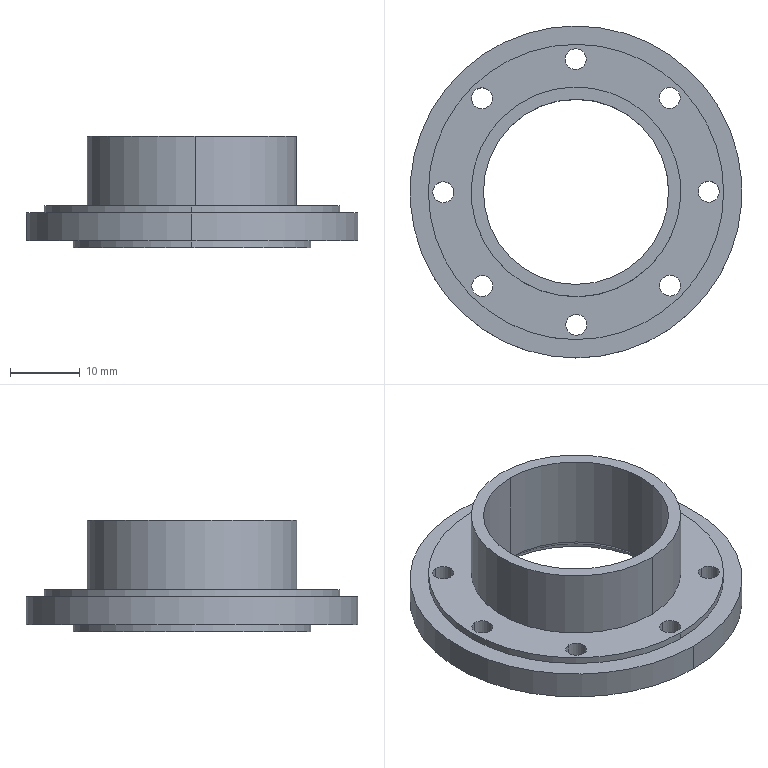Part | STEP file | 2026.6.15-Main Assembly图.sldasm-Part-105 | 1 solid | 36 faces | box 47.5 x 47.5 x 16 mm | volume 7161 mm3 | cylinder 28 | plane 6 | cone 2 | commonest cylinder face diameters 3 x16 30 x4 26.5 x2 34 x2 42.25 x2 47.5 x2
STEP:
#1=CARTESIAN_POINT('',(-1571.263,1411.006,3680.571));
#2=VERTEX_POINT('',#1);
#3=CARTESIAN_POINT('',(-1571.243,1437.506,3680.571));
#4=VERTEX_POINT('',#3);
#5=CARTESIAN_POINT('',(-1571.253,1424.256,3680.571));
#6=DIRECTION('',(0.,0.,-1.));
#7=DIRECTION('',(-0.0007664,-1.,0.));
#8=AXIS2_PLACEMENT_3D('',#5,#6,#7);
#9=CIRCLE('',#8,13.25);
#10=EDGE_CURVE('',#2,#4,#9,.T.);
#11=ORIENTED_EDGE('',*,*,#10,.F.);
#12=CARTESIAN_POINT('',(-1571.264,1410.006,3679.571));
#13=VERTEX_POINT('',#12);
#14=CARTESIAN_POINT('',(-1571.263,1411.006,3680.571));
#15=DIRECTION('',(-0.000542,-0.7071,-0.7071));
#16=VECTOR('',#15,1000.);
#17=LINE('',#14,#16);
#18=EDGE_CURVE('',#2,#13,#17,.T.);
#19=ORIENTED_EDGE('',*,*,#18,.T.);
#20=CARTESIAN_POINT('',(-1571.242,1438.506,3679.571));
#21=VERTEX_POINT('',#20);
#22=CARTESIAN_POINT('',(-1571.253,1424.256,3679.571));
#23=DIRECTION('',(0.,0.,1.));
#24=DIRECTION('',(-0.0007664,-1.,0.));
#25=AXIS2_PLACEMENT_3D('',#22,#23,#24);
#26=CIRCLE('',#25,14.25);
#27=EDGE_CURVE('',#21,#13,#26,.T.);
#28=ORIENTED_EDGE('',*,*,#27,.F.);
#29=CARTESIAN_POINT('',(-1571.243,1437.506,3680.571));
#30=DIRECTION('',(0.000542,0.7071,-0.7071));
#31=VECTOR('',#30,1000.);
#32=LINE('',#29,#31);
#33=EDGE_CURVE('',#4,#21,#32,.T.);
#34=ORIENTED_EDGE('',*,*,#33,.F.);
#35=EDGE_LOOP('',(#11,#19,#28,#34));
#36=FACE_OUTER_BOUND('',#35,.T.);
#37=CARTESIAN_POINT('',(-1571.253,1424.256,3680.571));
#38=DIRECTION('',(0.,0.,-1.));
#39=DIRECTION('',(0.0007664,1.,0.));
#40=AXIS2_PLACEMENT_3D('',#37,#38,#39);
#41=CONICAL_SURFACE('',#40,13.25,0.7854);
#42=ADVANCED_FACE('',(#36),#41,.F.);
#43=CARTESIAN_POINT('',(-1571.263,1411.006,3694.571));
#44=VERTEX_POINT('',#43);
#45=CARTESIAN_POINT('',(-1571.243,1437.506,3694.571));
#46=VERTEX_POINT('',#45);
#47=CARTESIAN_POINT('',(-1571.253,1424.256,3694.571));
#48=DIRECTION('',(0.,0.,-1.));
#49=DIRECTION('',(-0.0007664,-1.,0.));
#50=AXIS2_PLACEMENT_3D('',#47,#48,#49);
#51=CIRCLE('',#50,13.25);
#52=EDGE_CURVE('',#44,#46,#51,.T.);
#53=ORIENTED_EDGE('',*,*,#52,.F.);
#54=CARTESIAN_POINT('',(-1571.263,1411.006,3710.571));
#55=DIRECTION('',(0.,0.,-1.));
#56=VECTOR('',#55,1000.);
#57=LINE('',#54,#56);
#58=EDGE_CURVE('',#44,#2,#57,.T.);
#59=ORIENTED_EDGE('',*,*,#58,.T.);
#60=ORIENTED_EDGE('',*,*,#10,.T.);
#61=CARTESIAN_POINT('',(-1571.243,1437.506,3710.571));
#62=DIRECTION('',(0.,0.,-1.));
#63=VECTOR('',#62,1000.);
#64=LINE('',#61,#63);
#65=EDGE_CURVE('',#46,#4,#64,.T.);
#66=ORIENTED_EDGE('',*,*,#65,.F.);
#67=EDGE_LOOP('',(#53,#59,#60,#66));
#68=FACE_OUTER_BOUND('',#67,.T.);
#69=CARTESIAN_POINT('',(-1571.253,1424.256,3710.571));
#70=DIRECTION('',(0.,0.,-1.));
#71=DIRECTION('',(0.0007664,1.,0.));
#72=AXIS2_PLACEMENT_3D('',#69,#70,#71);
#73=CYLINDRICAL_SURFACE('',#72,13.25);
#74=ADVANCED_FACE('',(#68),#73,.F.);
#75=CARTESIAN_POINT('',(-1571.269,1403.131,3684.571));
#76=VERTEX_POINT('',#75);
#77=CARTESIAN_POINT('',(-1571.237,1445.381,3684.571));
#78=VERTEX_POINT('',#77);
#79=CARTESIAN_POINT('',(-1571.253,1424.256,3684.571));
#80=DIRECTION('',(0.,0.,1.));
#81=DIRECTION('',(0.002193,-1.,0.));
#82=AXIS2_PLACEMENT_3D('',#79,#80,#81);
#83=CIRCLE('',#82,21.125);
#84=EDGE_CURVE('',#76,#78,#83,.T.);
#85=ORIENTED_EDGE('',*,*,#84,.F.);
#86=CARTESIAN_POINT('',(-1571.269,1403.131,3683.571));
#87=VERTEX_POINT('',#86);
#88=CARTESIAN_POINT('',(-1571.269,1403.131,3684.571));
#89=DIRECTION('',(0.,0.,-1.));
#90=VECTOR('',#89,1000.);
#91=LINE('',#88,#90);
#92=EDGE_CURVE('',#76,#87,#91,.T.);
#93=ORIENTED_EDGE('',*,*,#92,.T.);
#94=CARTESIAN_POINT('',(-1571.237,1445.381,3683.571));
#95=VERTEX_POINT('',#94);
#96=CARTESIAN_POINT('',(-1571.253,1424.256,3683.571));
#97=DIRECTION('',(0.,0.,1.));
#98=DIRECTION('',(0.002193,-1.,0.));
#99=AXIS2_PLACEMENT_3D('',#96,#97,#98);
#100=CIRCLE('',#99,21.125);
#101=EDGE_CURVE('',#87,#95,#100,.T.);
#102=ORIENTED_EDGE('',*,*,#101,.T.);
#103=CARTESIAN_POINT('',(-1571.237,1445.381,3684.571));
#104=DIRECTION('',(0.,0.,-1.));
#105=VECTOR('',#104,1000.);
#106=LINE('',#103,#105);
#107=EDGE_CURVE('',#78,#95,#106,.T.);
#108=ORIENTED_EDGE('',*,*,#107,.F.);
#109=EDGE_LOOP('',(#85,#93,#102,#108));
#110=FACE_OUTER_BOUND('',#109,.T.);
#111=CARTESIAN_POINT('',(-1571.253,1424.256,3684.571));
#112=DIRECTION('',(0.,0.,-1.));
#113=DIRECTION('',(0.0007664,1.,0.));
#114=AXIS2_PLACEMENT_3D('',#111,#112,#113);
#115=CYLINDRICAL_SURFACE('',#114,21.125);
#116=ADVANCED_FACE('',(#110),#115,.T.);
#117=CARTESIAN_POINT('',(-1570.823,1409.262,3684.571));
#118=VERTEX_POINT('',#117);
#119=CARTESIAN_POINT('',(-1571.684,1439.25,3684.571));
#120=VERTEX_POINT('',#119);
#121=CARTESIAN_POINT('',(-1571.253,1424.256,3684.571));
#122=DIRECTION('',(0.,0.,1.));
#123=DIRECTION('',(0.02871,-0.9996,0.));
#124=AXIS2_PLACEMENT_3D('',#121,#122,#123);
#125=CIRCLE('',#124,15.);
#126=EDGE_CURVE('',#118,#120,#125,.T.);
#127=ORIENTED_EDGE('',*,*,#126,.T.);
#128=CARTESIAN_POINT('',(-1571.684,1439.25,3694.571));
#129=VERTEX_POINT('',#128);
#130=CARTESIAN_POINT('',(-1571.684,1439.25,3684.571));
#131=DIRECTION('',(0.,0.,1.));
#132=VECTOR('',#131,1000.);
#133=LINE('',#130,#132);
#134=EDGE_CURVE('',#120,#129,#133,.T.);
#135=ORIENTED_EDGE('',*,*,#134,.T.);
#136=CARTESIAN_POINT('',(-1570.823,1409.262,3694.571));
#137=VERTEX_POINT('',#136);
#138=CARTESIAN_POINT('',(-1571.253,1424.256,3694.571));
#139=DIRECTION('',(0.,0.,-1.));
#140=DIRECTION('',(0.02871,-0.9996,0.));
#141=AXIS2_PLACEMENT_3D('',#138,#139,#140);
#142=CIRCLE('',#141,15.);
#143=EDGE_CURVE('',#129,#137,#142,.T.);
#144=ORIENTED_EDGE('',*,*,#143,.T.);
#145=CARTESIAN_POINT('',(-1570.823,1409.262,3684.571));
#146=DIRECTION('',(0.,0.,1.));
#147=VECTOR('',#146,1000.);
#148=LINE('',#145,#147);
#149=EDGE_CURVE('',#118,#137,#148,.T.);
#150=ORIENTED_EDGE('',*,*,#149,.F.);
#151=EDGE_LOOP('',(#127,#135,#144,#150));
#152=FACE_OUTER_BOUND('',#151,.T.);
#153=CARTESIAN_POINT('',(-1571.253,1424.256,3684.571));
#154=DIRECTION('',(0.,0.,1.));
#155=DIRECTION('',(0.02871,-0.9996,0.));
#156=AXIS2_PLACEMENT_3D('',#153,#154,#155);
#157=CYLINDRICAL_SURFACE('',#156,15.);
#158=ADVANCED_FACE('',(#152),#157,.T.);
#159=CARTESIAN_POINT('',(-1571.294,1444.756,3684.571));
#160=VERTEX_POINT('',#159);
#161=CARTESIAN_POINT('',(-1571.296,1441.756,3684.571));
#162=VERTEX_POINT('',#161);
#163=CARTESIAN_POINT('',(-1571.295,1443.256,3684.571));
#164=DIRECTION('',(0.,0.,1.));
#165=DIRECTION('',(0.002193,-1.,0.));
#166=AXIS2_PLACEMENT_3D('',#163,#164,#165);
#167=CIRCLE('',#166,1.5);
#168=EDGE_CURVE('',#160,#162,#167,.T.);
#169=ORIENTED_EDGE('',*,*,#168,.T.);
#170=CARTESIAN_POINT('',(-1571.296,1441.756,3679.571));
#171=VERTEX_POINT('',#170);
#172=CARTESIAN_POINT('',(-1571.296,1441.756,3683.571));
#173=DIRECTION('',(0.,0.,-1.));
#174=VECTOR('',#173,1000.);
#175=LINE('',#172,#174);
#176=EDGE_CURVE('',#162,#171,#175,.T.);
#177=ORIENTED_EDGE('',*,*,#176,.T.);
#178=CARTESIAN_POINT('',(-1571.294,1444.756,3679.571));
#179=VERTEX_POINT('',#178);
#180=CARTESIAN_POINT('',(-1571.295,1443.256,3679.571));
#181=DIRECTION('',(0.,0.,1.));
#182=DIRECTION('',(0.002193,-1.,0.));
#183=AXIS2_PLACEMENT_3D('',#180,#181,#182);
#184=CIRCLE('',#183,1.5);
#185=EDGE_CURVE('',#179,#171,#184,.T.);
#186=ORIENTED_EDGE('',*,*,#185,.F.);
#187=CARTESIAN_POINT('',(-1571.294,1444.756,3683.571));
#188=DIRECTION('',(0.,0.,-1.));
#189=VECTOR('',#188,1000.);
#190=LINE('',#187,#189);
#191=EDGE_CURVE('',#160,#179,#190,.T.);
#192=ORIENTED_EDGE('',*,*,#191,.F.);
#193=EDGE_LOOP('',(#169,#177,#186,#192));
#194=FACE_OUTER_BOUND('',#193,.T.);
#195=CARTESIAN_POINT('',(-1571.295,1443.256,3683.571));
#196=DIRECTION('',(0.,0.,-1.));
#197=DIRECTION('',(0.0007664,1.,0.));
#198=AXIS2_PLACEMENT_3D('',#195,#196,#197);
#199=CYLINDRICAL_SURFACE('',#198,1.5);
#200=ADVANCED_FACE('',(#194),#199,.F.);
#201=CARTESIAN_POINT('',(-1571.235,1448.006,3683.571));
#202=VERTEX_POINT('',#201);
#203=CARTESIAN_POINT('',(-1571.271,1400.506,3683.571));
#204=VERTEX_POINT('',#203);
#205=CARTESIAN_POINT('',(-1571.253,1424.256,3683.571));
#206=DIRECTION('',(0.,0.,-1.));
#207=DIRECTION('',(0.002193,-1.,0.));
#208=AXIS2_PLACEMENT_3D('',#205,#206,#207);
#209=CIRCLE('',#208,23.75);
#210=EDGE_CURVE('',#202,#204,#209,.T.);
#211=ORIENTED_EDGE('',*,*,#210,.T.);
#212=CARTESIAN_POINT('',(-1571.271,1400.506,3679.571));
#213=VERTEX_POINT('',#212);
#214=CARTESIAN_POINT('',(-1571.271,1400.506,3683.571));
#215=DIRECTION('',(0.,0.,-1.));
#216=VECTOR('',#215,1000.);
#217=LINE('',#214,#216);
#218=EDGE_CURVE('',#204,#213,#217,.T.);
#219=ORIENTED_EDGE('',*,*,#218,.T.);
#220=CARTESIAN_POINT('',(-1571.235,1448.006,3679.571));
#221=VERTEX_POINT('',#220);
#222=CARTESIAN_POINT('',(-1571.253,1424.256,3679.571));
#223=DIRECTION('',(0.,0.,-1.));
#224=DIRECTION('',(0.002193,-1.,0.));
#225=AXIS2_PLACEMENT_3D('',#222,#223,#224);
#226=CIRCLE('',#225,23.75);
#227=EDGE_CURVE('',#221,#213,#226,.T.);
#228=ORIENTED_EDGE('',*,*,#227,.F.);
#229=CARTESIAN_POINT('',(-1571.235,1448.006,3683.571));
#230=DIRECTION('',(0.,0.,-1.));
#231=VECTOR('',#230,1000.);
#232=LINE('',#229,#231);
#233=EDGE_CURVE('',#202,#221,#232,.T.);
#234=ORIENTED_EDGE('',*,*,#233,.F.);
#235=EDGE_LOOP('',(#211,#219,#228,#234));
#236=FACE_OUTER_BOUND('',#235,.T.);
#237=CARTESIAN_POINT('',(-1571.253,1424.256,3683.571));
#238=DIRECTION('',(0.,0.,-1.));
#239=DIRECTION('',(0.0007664,1.,0.));
#240=AXIS2_PLACEMENT_3D('',#237,#238,#239);
#241=CYLINDRICAL_SURFACE('',#240,23.75);
#242=ADVANCED_FACE('',(#236),#241,.T.);
#243=CARTESIAN_POINT('',(-1571.21,1406.756,3684.571));
#244=VERTEX_POINT('',#243);
#245=CARTESIAN_POINT('',(-1571.213,1403.756,3684.571));
#246=VERTEX_POINT('',#245);
#247=CARTESIAN_POINT('',(-1571.211,1405.256,3684.571));
#248=DIRECTION('',(0.,0.,1.));
#249=DIRECTION('',(0.002193,-1.,0.));
#250=AXIS2_PLACEMENT_3D('',#247,#248,#249);
#251=CIRCLE('',#250,1.5);
#252=EDGE_CURVE('',#244,#246,#251,.T.);
#253=ORIENTED_EDGE('',*,*,#252,.T.);
#254=CARTESIAN_POINT('',(-1571.213,1403.756,3679.571));
#255=VERTEX_POINT('',#254);
#256=CARTESIAN_POINT('',(-1571.213,1403.756,3683.571));
#257=DIRECTION('',(0.,0.,-1.));
#258=VECTOR('',#257,1000.);
#259=LINE('',#256,#258);
#260=EDGE_CURVE('',#246,#255,#259,.T.);
#261=ORIENTED_EDGE('',*,*,#260,.T.);
#262=CARTESIAN_POINT('',(-1571.21,1406.756,3679.571));
#263=VERTEX_POINT('',#262);
#264=CARTESIAN_POINT('',(-1571.211,1405.256,3679.571));
#265=DIRECTION('',(0.,0.,1.));
#266=DIRECTION('',(0.002193,-1.,0.));
#267=AXIS2_PLACEMENT_3D('',#264,#265,#266);
#268=CIRCLE('',#267,1.5);
#269=EDGE_CURVE('',#263,#255,#268,.T.);
#270=ORIENTED_EDGE('',*,*,#269,.F.);
#271=CARTESIAN_POINT('',(-1571.21,1406.756,3683.571));
#272=DIRECTION('',(0.,0.,-1.));
#273=VECTOR('',#272,1000.);
#274=LINE('',#271,#273);
#275=EDGE_CURVE('',#244,#263,#274,.T.);
#276=ORIENTED_EDGE('',*,*,#275,.F.);
#277=EDGE_LOOP('',(#253,#261,#270,#276));
#278=FACE_OUTER_BOUND('',#277,.T.);
#279=CARTESIAN_POINT('',(-1571.211,1405.256,3683.571));
#280=DIRECTION('',(0.,0.,-1.));
#281=DIRECTION('',(0.0007664,1.,0.));
#282=AXIS2_PLACEMENT_3D('',#279,#280,#281);
#283=CYLINDRICAL_SURFACE('',#282,1.5);
#284=ADVANCED_FACE('',(#278),#283,.F.);
#285=CARTESIAN_POINT('',(-1557.788,1412.35,3684.571));
#286=VERTEX_POINT('',#285);
#287=CARTESIAN_POINT('',(-1557.79,1409.35,3684.571));
#288=VERTEX_POINT('',#287);
#289=CARTESIAN_POINT('',(-1557.789,1410.85,3684.571));
#290=DIRECTION('',(0.,0.,1.));
#291=DIRECTION('',(0.002193,-1.,0.));
#292=AXIS2_PLACEMENT_3D('',#289,#290,#291);
#293=CIRCLE('',#292,1.5);
#294=EDGE_CURVE('',#286,#288,#293,.T.);
#295=ORIENTED_EDGE('',*,*,#294,.T.);
#296=CARTESIAN_POINT('',(-1557.79,1409.35,3679.571));
#297=VERTEX_POINT('',#296);
#298=CARTESIAN_POINT('',(-1557.79,1409.35,3683.571));
#299=DIRECTION('',(0.,0.,-1.));
#300=VECTOR('',#299,1000.);
#301=LINE('',#298,#300);
#302=EDGE_CURVE('',#288,#297,#301,.T.);
#303=ORIENTED_EDGE('',*,*,#302,.T.);
#304=CARTESIAN_POINT('',(-1557.788,1412.35,3679.571));
#305=VERTEX_POINT('',#304);
#306=CARTESIAN_POINT('',(-1557.789,1410.85,3679.571));
#307=DIRECTION('',(0.,0.,1.));
#308=DIRECTION('',(0.002193,-1.,0.));
#309=AXIS2_PLACEMENT_3D('',#306,#307,#308);
#310=CIRCLE('',#309,1.5);
#311=EDGE_CURVE('',#305,#297,#310,.T.);
#312=ORIENTED_EDGE('',*,*,#311,.F.);
#313=CARTESIAN_POINT('',(-1557.788,1412.35,3683.571));
#314=DIRECTION('',(0.,0.,-1.));
#315=VECTOR('',#314,1000.);
#316=LINE('',#313,#315);
#317=EDGE_CURVE('',#286,#305,#316,.T.);
#318=ORIENTED_EDGE('',*,*,#317,.F.);
#319=EDGE_LOOP('',(#295,#303,#312,#318));
#320=FACE_OUTER_BOUND('',#319,.T.);
#321=CARTESIAN_POINT('',(-1557.789,1410.85,3683.571));
#322=DIRECTION('',(0.,0.,-1.));
#323=DIRECTION('',(0.0007664,1.,0.));
#324=AXIS2_PLACEMENT_3D('',#321,#322,#323);
#325=CYLINDRICAL_SURFACE('',#324,1.5);
#326=ADVANCED_FACE('',(#320),#325,.F.);
#327=CARTESIAN_POINT('',(-1584.658,1412.291,3684.571));
#328=VERTEX_POINT('',#327);
#329=CARTESIAN_POINT('',(-1584.66,1409.291,3684.571));
#330=VERTEX_POINT('',#329);
#331=CARTESIAN_POINT('',(-1584.659,1410.791,3684.571));
#332=DIRECTION('',(0.,0.,1.));
#333=DIRECTION('',(0.002193,-1.,0.));
#334=AXIS2_PLACEMENT_3D('',#331,#332,#333);
#335=CIRCLE('',#334,1.5);
#336=EDGE_CURVE('',#328,#330,#335,.T.);
#337=ORIENTED_EDGE('',*,*,#336,.T.);
#338=CARTESIAN_POINT('',(-1584.66,1409.291,3679.571));
#339=VERTEX_POINT('',#338);
#340=CARTESIAN_POINT('',(-1584.66,1409.291,3683.571));
#341=DIRECTION('',(0.,0.,-1.));
#342=VECTOR('',#341,1000.);
#343=LINE('',#340,#342);
#344=EDGE_CURVE('',#330,#339,#343,.T.);
#345=ORIENTED_EDGE('',*,*,#344,.T.);
#346=CARTESIAN_POINT('',(-1584.658,1412.291,3679.571));
#347=VERTEX_POINT('',#346);
#348=CARTESIAN_POINT('',(-1584.659,1410.791,3679.571));
#349=DIRECTION('',(0.,0.,1.));
#350=DIRECTION('',(0.002193,-1.,0.));
#351=AXIS2_PLACEMENT_3D('',#348,#349,#350);
#352=CIRCLE('',#351,1.5);
#353=EDGE_CURVE('',#347,#339,#352,.T.);
#354=ORIENTED_EDGE('',*,*,#353,.F.);
#355=CARTESIAN_POINT('',(-1584.658,1412.291,3683.571));
#356=DIRECTION('',(0.,0.,-1.));
#357=VECTOR('',#356,1000.);
#358=LINE('',#355,#357);
#359=EDGE_CURVE('',#328,#347,#358,.T.);
#360=ORIENTED_EDGE('',*,*,#359,.F.);
#361=EDGE_LOOP('',(#337,#345,#354,#360));
#362=FACE_OUTER_BOUND('',#361,.T.);
#363=CARTESIAN_POINT('',(-1584.659,1410.791,3683.571));
#364=DIRECTION('',(0.,0.,-1.));
#365=DIRECTION('',(0.0007664,1.,0.));
#366=AXIS2_PLACEMENT_3D('',#363,#364,#365);
#367=CYLINDRICAL_SURFACE('',#366,1.5);
#368=ADVANCED_FACE('',(#362),#367,.F.);
#369=CARTESIAN_POINT('',(-1552.252,1425.798,3684.571));
#370=VERTEX_POINT('',#369);
#371=CARTESIAN_POINT('',(-1552.254,1422.798,3684.571));
#372=VERTEX_POINT('',#371);
#373=CARTESIAN_POINT('',(-1552.253,1424.298,3684.571));
#374=DIRECTION('',(0.,0.,1.));
#375=DIRECTION('',(0.002193,-1.,0.));
#376=AXIS2_PLACEMENT_3D('',#373,#374,#375);
#377=CIRCLE('',#376,1.5);
#378=EDGE_CURVE('',#370,#372,#377,.T.);
#379=ORIENTED_EDGE('',*,*,#378,.T.);
#380=CARTESIAN_POINT('',(-1552.254,1422.798,3679.571));
#381=VERTEX_POINT('',#380);
#382=CARTESIAN_POINT('',(-1552.254,1422.798,3683.571));
#383=DIRECTION('',(0.,0.,-1.));
#384=VECTOR('',#383,1000.);
#385=LINE('',#382,#384);
#386=EDGE_CURVE('',#372,#381,#385,.T.);
#387=ORIENTED_EDGE('',*,*,#386,.T.);
#388=CARTESIAN_POINT('',(-1552.252,1425.798,3679.571));
#389=VERTEX_POINT('',#388);
#390=CARTESIAN_POINT('',(-1552.253,1424.298,3679.571));
#391=DIRECTION('',(0.,0.,1.));
#392=DIRECTION('',(0.002193,-1.,0.));
#393=AXIS2_PLACEMENT_3D('',#390,#391,#392);
#394=CIRCLE('',#393,1.5);
#395=EDGE_CURVE('',#389,#381,#394,.T.);
#396=ORIENTED_EDGE('',*,*,#395,.F.);
#397=CARTESIAN_POINT('',(-1552.252,1425.798,3683.571));
#398=DIRECTION('',(0.,0.,-1.));
#399=VECTOR('',#398,1000.);
#400=LINE('',#397,#399);
#401=EDGE_CURVE('',#370,#389,#400,.T.);
#402=ORIENTED_EDGE('',*,*,#401,.F.);
#403=EDGE_LOOP('',(#379,#387,#396,#402));
#404=FACE_OUTER_BOUND('',#403,.T.);
#405=CARTESIAN_POINT('',(-1552.253,1424.298,3683.571));
#406=DIRECTION('',(0.,0.,-1.));
#407=DIRECTION('',(0.0007664,1.,0.));
#408=AXIS2_PLACEMENT_3D('',#405,#406,#407);
#409=CYLINDRICAL_SURFACE('',#408,1.5);
#410=ADVANCED_FACE('',(#404),#409,.F.);
#411=CARTESIAN_POINT('',(-1590.252,1425.714,3684.571));
#412=VERTEX_POINT('',#411);
#413=CARTESIAN_POINT('',(-1590.254,1422.714,3684.571));
#414=VERTEX_POINT('',#413);
#415=CARTESIAN_POINT('',(-1590.253,1424.214,3684.571));
#416=DIRECTION('',(0.,0.,1.));
#417=DIRECTION('',(0.002193,-1.,0.));
#418=AXIS2_PLACEMENT_3D('',#415,#416,#417);
#419=CIRCLE('',#418,1.5);
#420=EDGE_CURVE('',#412,#414,#419,.T.);
#421=ORIENTED_EDGE('',*,*,#420,.T.);
#422=CARTESIAN_POINT('',(-1590.254,1422.714,3679.571));
#423=VERTEX_POINT('',#422);
#424=CARTESIAN_POINT('',(-1590.254,1422.714,3683.571));
#425=DIRECTION('',(0.,0.,-1.));
#426=VECTOR('',#425,1000.);
#427=LINE('',#424,#426);
#428=EDGE_CURVE('',#414,#423,#427,.T.);
#429=ORIENTED_EDGE('',*,*,#428,.T.);
#430=CARTESIAN_POINT('',(-1590.252,1425.714,3679.571));
#431=VERTEX_POINT('',#430);
#432=CARTESIAN_POINT('',(-1590.253,1424.214,3679.571));
#433=DIRECTION('',(0.,0.,1.));
#434=DIRECTION('',(0.002193,-1.,0.));
#435=AXIS2_PLACEMENT_3D('',#432,#433,#434);
#436=CIRCLE('',#435,1.5);
#437=EDGE_CURVE('',#431,#423,#436,.T.);
#438=ORIENTED_EDGE('',*,*,#437,.F.);
#439=CARTESIAN_POINT('',(-1590.252,1425.714,3683.571));
#440=DIRECTION('',(0.,0.,-1.));
#441=VECTOR('',#440,1000.);
#442=LINE('',#439,#441);
#443=EDGE_CURVE('',#412,#431,#442,.T.);
#444=ORIENTED_EDGE('',*,*,#443,.F.);
#445=EDGE_LOOP('',(#421,#429,#438,#444));
#446=FACE_OUTER_BOUND('',#445,.T.);
#447=CARTESIAN_POINT('',(-1590.253,1424.214,3683.571));
#448=DIRECTION('',(0.,0.,-1.));
#449=DIRECTION('',(0.0007664,1.,0.));
#450=AXIS2_PLACEMENT_3D('',#447,#448,#449);
#451=CYLINDRICAL_SURFACE('',#450,1.5);
#452=ADVANCED_FACE('',(#446),#451,.F.);
#453=CARTESIAN_POINT('',(-1557.846,1439.22,3684.571));
#454=VERTEX_POINT('',#453);
#455=CARTESIAN_POINT('',(-1557.849,1436.22,3684.571));
#456=VERTEX_POINT('',#455);
#457=CARTESIAN_POINT('',(-1557.848,1437.72,3684.571));
#458=DIRECTION('',(0.,0.,1.));
#459=DIRECTION('',(0.002193,-1.,0.));
#460=AXIS2_PLACEMENT_3D('',#457,#458,#459);
#461=CIRCLE('',#460,1.5);
#462=EDGE_CURVE('',#454,#456,#461,.T.);
#463=ORIENTED_EDGE('',*,*,#462,.T.);
#464=CARTESIAN_POINT('',(-1557.849,1436.22,3679.571));
#465=VERTEX_POINT('',#464);
#466=CARTESIAN_POINT('',(-1557.849,1436.22,3683.571));
#467=DIRECTION('',(0.,0.,-1.));
#468=VECTOR('',#467,1000.);
#469=LINE('',#466,#468);
#470=EDGE_CURVE('',#456,#465,#469,.T.);
#471=ORIENTED_EDGE('',*,*,#470,.T.);
#472=CARTESIAN_POINT('',(-1557.846,1439.22,3679.571));
#473=VERTEX_POINT('',#472);
#474=CARTESIAN_POINT('',(-1557.848,1437.72,3679.571));
#475=DIRECTION('',(0.,0.,1.));
#476=DIRECTION('',(0.002193,-1.,0.));
#477=AXIS2_PLACEMENT_3D('',#474,#475,#476);
#478=CIRCLE('',#477,1.5);
#479=EDGE_CURVE('',#473,#465,#478,.T.);
#480=ORIENTED_EDGE('',*,*,#479,.F.);
#481=CARTESIAN_POINT('',(-1557.846,1439.22,3683.571));
#482=DIRECTION('',(0.,0.,-1.));
#483=VECTOR('',#482,1000.);
#484=LINE('',#481,#483);
#485=EDGE_CURVE('',#454,#473,#484,.T.);
#486=ORIENTED_EDGE('',*,*,#485,.F.);
#487=EDGE_LOOP('',(#463,#471,#480,#486));
#488=FACE_OUTER_BOUND('',#487,.T.);
#489=CARTESIAN_POINT('',(-1557.848,1437.72,3683.571));
#490=DIRECTION('',(0.,0.,-1.));
#491=DIRECTION('',(0.0007664,1.,0.));
#492=AXIS2_PLACEMENT_3D('',#489,#490,#491);
#493=CYLINDRICAL_SURFACE('',#492,1.5);
#494=ADVANCED_FACE('',(#488),#493,.F.);
#495=CARTESIAN_POINT('',(-1584.716,1439.161,3684.571));
#496=VERTEX_POINT('',#495);
#497=CARTESIAN_POINT('',(-1584.719,1436.161,3684.571));
#498=VERTEX_POINT('',#497);
#499=CARTESIAN_POINT('',(-1584.718,1437.661,3684.571));
#500=DIRECTION('',(0.,0.,1.));
#501=DIRECTION('',(0.002193,-1.,0.));
#502=AXIS2_PLACEMENT_3D('',#499,#500,#501);
#503=CIRCLE('',#502,1.5);
#504=EDGE_CURVE('',#496,#498,#503,.T.);
#505=ORIENTED_EDGE('',*,*,#504,.T.);
#506=CARTESIAN_POINT('',(-1584.719,1436.161,3679.571));
#507=VERTEX_POINT('',#506);
#508=CARTESIAN_POINT('',(-1584.719,1436.161,3683.571));
#509=DIRECTION('',(0.,0.,-1.));
#510=VECTOR('',#509,1000.);
#511=LINE('',#508,#510);
#512=EDGE_CURVE('',#498,#507,#511,.T.);
#513=ORIENTED_EDGE('',*,*,#512,.T.);
#514=CARTESIAN_POINT('',(-1584.716,1439.161,3679.571));
#515=VERTEX_POINT('',#514);
#516=CARTESIAN_POINT('',(-1584.718,1437.661,3679.571));
#517=DIRECTION('',(0.,0.,1.));
#518=DIRECTION('',(0.002193,-1.,0.));
#519=AXIS2_PLACEMENT_3D('',#516,#517,#518);
#520=CIRCLE('',#519,1.5);
#521=EDGE_CURVE('',#515,#507,#520,.T.);
#522=ORIENTED_EDGE('',*,*,#521,.F.);
#523=CARTESIAN_POINT('',(-1584.716,1439.161,3683.571));
#524=DIRECTION('',(0.,0.,-1.));
#525=VECTOR('',#524,1000.);
#526=LINE('',#523,#525);
#527=EDGE_CURVE('',#496,#515,#526,.T.);
#528=ORIENTED_EDGE('',*,*,#527,.F.);
#529=EDGE_LOOP('',(#505,#513,#522,#528));
#530=FACE_OUTER_BOUND('',#529,.T.);
#531=CARTESIAN_POINT('',(-1584.718,1437.661,3683.571));
#532=DIRECTION('',(0.,0.,-1.));
#533=DIRECTION('',(0.0007664,1.,0.));
#534=AXIS2_PLACEMENT_3D('',#531,#532,#533);
#535=CYLINDRICAL_SURFACE('',#534,1.5);
#536=ADVANCED_FACE('',(#530),#535,.F.);
#537=CARTESIAN_POINT('',(-1571.242,1439.256,3679.571));
#538=VERTEX_POINT('',#537);
#539=CARTESIAN_POINT('',(-1571.265,1409.256,3679.571));
#540=VERTEX_POINT('',#539);
#541=CARTESIAN_POINT('',(-1571.253,1424.256,3679.571));
#542=DIRECTION('',(0.,0.,1.));
#543=DIRECTION('',(-0.0007664,-1.,0.));
#544=AXIS2_PLACEMENT_3D('',#541,#542,#543);
#545=CIRCLE('',#544,15.);
#546=EDGE_CURVE('',#538,#540,#545,.T.);
#547=ORIENTED_EDGE('',*,*,#546,.T.);
#548=CARTESIAN_POINT('',(-1571.265,1409.256,3678.571));
#549=VERTEX_POINT('',#548);
#550=CARTESIAN_POINT('',(-1571.265,1409.256,3679.571));
#551=DIRECTION('',(0.,0.,-1.));
#552=VECTOR('',#551,1000.);
#553=LINE('',#550,#552);
#554=EDGE_CURVE('',#540,#549,#553,.T.);
#555=ORIENTED_EDGE('',*,*,#554,.T.);
#556=CARTESIAN_POINT('',(-1571.242,1439.256,3678.571));
#557=VERTEX_POINT('',#556);
#558=CARTESIAN_POINT('',(-1571.253,1424.256,3678.571));
#559=DIRECTION('',(0.,0.,1.));
#560=DIRECTION('',(-0.0007664,-1.,0.));
#561=AXIS2_PLACEMENT_3D('',#558,#559,#560);
#562=CIRCLE('',#561,15.);
#563=EDGE_CURVE('',#557,#549,#562,.T.);
#564=ORIENTED_EDGE('',*,*,#563,.F.);
#565=CARTESIAN_POINT('',(-1571.242,1439.256,3679.571));
#566=DIRECTION('',(0.,0.,-1.));
#567=VECTOR('',#566,1000.);
#568=LINE('',#565,#567);
#569=EDGE_CURVE('',#538,#557,#568,.T.);
#570=ORIENTED_EDGE('',*,*,#569,.F.);
#571=EDGE_LOOP('',(#547,#555,#564,#570));
#572=FACE_OUTER_BOUND('',#571,.T.);
#573=CARTESIAN_POINT('',(-1571.253,1424.256,3679.571));
#574=DIRECTION('',(0.,0.,-1.));
#575=DIRECTION('',(0.0007664,1.,0.));
#576=AXIS2_PLACEMENT_3D('',#573,#574,#575);
#577=CYLINDRICAL_SURFACE('',#576,15.);
#578=ADVANCED_FACE('',(#572),#577,.F.);
#579=CARTESIAN_POINT('',(-1571.266,1407.256,3679.571));
#580=VERTEX_POINT('',#579);
#581=CARTESIAN_POINT('',(-1571.24,1441.256,3679.571));
#582=VERTEX_POINT('',#581);
#583=CARTESIAN_POINT('',(-1571.253,1424.256,3679.571));
#584=DIRECTION('',(0.,0.,1.));
#585=DIRECTION('',(0.002193,-1.,0.));
#586=AXIS2_PLACEMENT_3D('',#583,#584,#585);
#587=CIRCLE('',#586,17.);
#588=EDGE_CURVE('',#580,#582,#587,.T.);
#589=ORIENTED_EDGE('',*,*,#588,.F.);
#590=CARTESIAN_POINT('',(-1571.266,1407.256,3678.571));
#591=VERTEX_POINT('',#590);
#592=CARTESIAN_POINT('',(-1571.266,1407.256,3679.571));
#593=DIRECTION('',(0.,0.,-1.));
#594=VECTOR('',#593,1000.);
#595=LINE('',#592,#594);
#596=EDGE_CURVE('',#580,#591,#595,.T.);
#597=ORIENTED_EDGE('',*,*,#596,.T.);
#598=CARTESIAN_POINT('',(-1571.24,1441.256,3678.571));
#599=VERTEX_POINT('',#598);
#600=CARTESIAN_POINT('',(-1571.253,1424.256,3678.571));
#601=DIRECTION('',(0.,0.,1.));
#602=DIRECTION('',(0.002193,-1.,0.));
#603=AXIS2_PLACEMENT_3D('',#600,#601,#602);
#604=CIRCLE('',#603,17.);
#605=EDGE_CURVE('',#591,#599,#604,.T.);
#606=ORIENTED_EDGE('',*,*,#605,.T.);
#607=CARTESIAN_POINT('',(-1571.24,1441.256,3679.571));
#608=DIRECTION('',(0.,0.,-1.));
#609=VECTOR('',#608,1000.);
#610=LINE('',#607,#609);
#611=EDGE_CURVE('',#582,#599,#610,.T.);
#612=ORIENTED_EDGE('',*,*,#611,.F.);
#613=EDGE_LOOP('',(#589,#597,#606,#612));
#614=FACE_OUTER_BOUND('',#613,.T.);
#615=CARTESIAN_POINT('',(-1571.253,1424.256,3679.571));
#616=DIRECTION('',(0.,0.,-1.));
#617=DIRECTION('',(0.0007664,1.,0.));
#618=AXIS2_PLACEMENT_3D('',#615,#616,#617);
#619=CYLINDRICAL_SURFACE('',#618,17.);
#620=ADVANCED_FACE('',(#614),#619,.T.);
#621=ORIENTED_EDGE('',*,*,#596,.F.);
#622=CARTESIAN_POINT('',(-1571.253,1424.256,3679.571));
#623=DIRECTION('',(0.,0.,1.));
#624=DIRECTION('',(0.002193,-1.,0.));
#625=AXIS2_PLACEMENT_3D('',#622,#623,#624);
#626=CIRCLE('',#625,17.);
#627=EDGE_CURVE('',#582,#580,#626,.T.);
#628=ORIENTED_EDGE('',*,*,#627,.F.);
#629=ORIENTED_EDGE('',*,*,#611,.T.);
#630=CARTESIAN_POINT('',(-1571.253,1424.256,3678.571));
#631=DIRECTION('',(0.,0.,1.));
#632=DIRECTION('',(0.002193,-1.,0.));
#633=AXIS2_PLACEMENT_3D('',#630,#631,#632);
#634=CIRCLE('',#633,17.);
#635=EDGE_CURVE('',#599,#591,#634,.T.);
#636=ORIENTED_EDGE('',*,*,#635,.T.);
#637=EDGE_LOOP('',(#621,#628,#629,#636));
#638=FACE_OUTER_BOUND('',#637,.T.);
#639=CARTESIAN_POINT('',(-1571.253,1424.256,3679.571));
#640=DIRECTION('',(0.,0.,-1.));
#641=DIRECTION('',(0.0007664,1.,0.));
#642=AXIS2_PLACEMENT_3D('',#639,#640,#641);
#643=CYLINDRICAL_SURFACE('',#642,17.);
#644=ADVANCED_FACE('',(#638),#643,.T.);
#645=ORIENTED_EDGE('',*,*,#554,.F.);
#646=CARTESIAN_POINT('',(-1571.253,1424.256,3679.571));
#647=DIRECTION('',(0.,0.,1.));
#648=DIRECTION('',(-0.0007664,-1.,0.));
#649=AXIS2_PLACEMENT_3D('',#646,#647,#648);
#650=CIRCLE('',#649,15.);
#651=EDGE_CURVE('',#540,#538,#650,.T.);
#652=ORIENTED_EDGE('',*,*,#651,.T.);
#653=ORIENTED_EDGE('',*,*,#569,.T.);
#654=CARTESIAN_POINT('',(-1571.253,1424.256,3678.571));
#655=DIRECTION('',(0.,0.,1.));
#656=DIRECTION('',(-0.0007664,-1.,0.));
#657=AXIS2_PLACEMENT_3D('',#654,#655,#656);
#658=CIRCLE('',#657,15.);
#659=EDGE_CURVE('',#549,#557,#658,.T.);
#660=ORIENTED_EDGE('',*,*,#659,.F.);
#661=EDGE_LOOP('',(#645,#652,#653,#660));
#662=FACE_OUTER_BOUND('',#661,.T.);
#663=CARTESIAN_POINT('',(-1571.253,1424.256,3679.571));
#664=DIRECTION('',(0.,0.,-1.));
#665=DIRECTION('',(0.0007664,1.,0.));
#666=AXIS2_PLACEMENT_3D('',#663,#664,#665);
#667=CYLINDRICAL_SURFACE('',#666,15.);
#668=ADVANCED_FACE('',(#662),#667,.F.);
#669=ORIENTED_EDGE('',*,*,#635,.F.);
#670=ORIENTED_EDGE('',*,*,#605,.F.);
#671=EDGE_LOOP('',(#669,#670));
#672=FACE_OUTER_BOUND('',#671,.T.);
#673=ORIENTED_EDGE('',*,*,#563,.T.);
#674=ORIENTED_EDGE('',*,*,#659,.T.);
#675=EDGE_LOOP('',(#673,#674));
#676=FACE_BOUND('',#675,.T.);
#677=CARTESIAN_POINT('',(-1571.253,1424.256,3678.571));
#678=DIRECTION('',(0.,0.,1.));
#679=DIRECTION('',(-0.0007664,-1.,0.));
#680=AXIS2_PLACEMENT_3D('',#677,#678,#679);
#681=PLANE('',#680);
#682=ADVANCED_FACE('',(#672,#676),#681,.F.);
#683=ORIENTED_EDGE('',*,*,#27,.T.);
#684=CARTESIAN_POINT('',(-1571.253,1424.256,3679.571));
#685=DIRECTION('',(0.,0.,1.));
#686=DIRECTION('',(-0.0007664,-1.,0.));
#687=AXIS2_PLACEMENT_3D('',#684,#685,#686);
#688=CIRCLE('',#687,14.25);
#689=EDGE_CURVE('',#13,#21,#688,.T.);
#690=ORIENTED_EDGE('',*,*,#689,.T.);
#691=EDGE_LOOP('',(#683,#690));
#692=FACE_BOUND('',#691,.T.);
#693=ORIENTED_EDGE('',*,*,#546,.F.);
#694=ORIENTED_EDGE('',*,*,#651,.F.);
#695=EDGE_LOOP('',(#693,#694));
#696=FACE_OUTER_BOUND('',#695,.T.);
#697=CARTESIAN_POINT('',(-1571.232,1414.756,3679.571));
#698=DIRECTION('',(0.,0.,1.));
#699=DIRECTION('',(-0.0007664,-1.,0.));
#700=AXIS2_PLACEMENT_3D('',#697,#698,#699);
#701=PLANE('',#700);
#702=ADVANCED_FACE('',(#692,#696),#701,.F.);
#703=ORIENTED_EDGE('',*,*,#512,.F.);
#704=CARTESIAN_POINT('',(-1584.718,1437.661,3684.571));
#705=DIRECTION('',(0.,0.,1.));
#706=DIRECTION('',(0.002193,-1.,0.));
#707=AXIS2_PLACEMENT_3D('',#704,#705,#706);
#708=CIRCLE('',#707,1.5);
#709=EDGE_CURVE('',#498,#496,#708,.T.);
#710=ORIENTED_EDGE('',*,*,#709,.T.);
#711=ORIENTED_EDGE('',*,*,#527,.T.);
#712=CARTESIAN_POINT('',(-1584.718,1437.661,3679.571));
#713=DIRECTION('',(0.,0.,1.));
#714=DIRECTION('',(0.002193,-1.,0.));
#715=AXIS2_PLACEMENT_3D('',#712,#713,#714);
#716=CIRCLE('',#715,1.5);
#717=EDGE_CURVE('',#507,#515,#716,.T.);
#718=ORIENTED_EDGE('',*,*,#717,.F.);
#719=EDGE_LOOP('',(#703,#710,#711,#718));
#720=FACE_OUTER_BOUND('',#719,.T.);
#721=CARTESIAN_POINT('',(-1584.718,1437.661,3683.571));
#722=DIRECTION('',(0.,0.,-1.));
#723=DIRECTION('',(0.0007664,1.,0.));
#724=AXIS2_PLACEMENT_3D('',#721,#722,#723);
#725=CYLINDRICAL_SURFACE('',#724,1.5);
#726=ADVANCED_FACE('',(#720),#725,.F.);
#727=ORIENTED_EDGE('',*,*,#470,.F.);
#728=CARTESIAN_POINT('',(-1557.848,1437.72,3684.571));
#729=DIRECTION('',(0.,0.,1.));
#730=DIRECTION('',(0.002193,-1.,0.));
#731=AXIS2_PLACEMENT_3D('',#728,#729,#730);
#732=CIRCLE('',#731,1.5);
#733=EDGE_CURVE('',#456,#454,#732,.T.);
#734=ORIENTED_EDGE('',*,*,#733,.T.);
#735=ORIENTED_EDGE('',*,*,#485,.T.);
#736=CARTESIAN_POINT('',(-1557.848,1437.72,3679.571));
#737=DIRECTION('',(0.,0.,1.));
#738=DIRECTION('',(0.002193,-1.,0.));
#739=AXIS2_PLACEMENT_3D('',#736,#737,#738);
#740=CIRCLE('',#739,1.5);
#741=EDGE_CURVE('',#465,#473,#740,.T.);
#742=ORIENTED_EDGE('',*,*,#741,.F.);
#743=EDGE_LOOP('',(#727,#734,#735,#742));
#744=FACE_OUTER_BOUND('',#743,.T.);
#745=CARTESIAN_POINT('',(-1557.848,1437.72,3683.571));
#746=DIRECTION('',(0.,0.,-1.));
#747=DIRECTION('',(0.0007664,1.,0.));
#748=AXIS2_PLACEMENT_3D('',#745,#746,#747);
#749=CYLINDRICAL_SURFACE('',#748,1.5);
#750=ADVANCED_FACE('',(#744),#749,.F.);
#751=ORIENTED_EDGE('',*,*,#428,.F.);
#752=CARTESIAN_POINT('',(-1590.253,1424.214,3684.571));
#753=DIRECTION('',(0.,0.,1.));
#754=DIRECTION('',(0.002193,-1.,0.));
#755=AXIS2_PLACEMENT_3D('',#752,#753,#754);
#756=CIRCLE('',#755,1.5);
#757=EDGE_CURVE('',#414,#412,#756,.T.);
#758=ORIENTED_EDGE('',*,*,#757,.T.);
#759=ORIENTED_EDGE('',*,*,#443,.T.);
#760=CARTESIAN_POINT('',(-1590.253,1424.214,3679.571));
#761=DIRECTION('',(0.,0.,1.));
#762=DIRECTION('',(0.002193,-1.,0.));
#763=AXIS2_PLACEMENT_3D('',#760,#761,#762);
#764=CIRCLE('',#763,1.5);
#765=EDGE_CURVE('',#423,#431,#764,.T.);
#766=ORIENTED_EDGE('',*,*,#765,.F.);
#767=EDGE_LOOP('',(#751,#758,#759,#766));
#768=FACE_OUTER_BOUND('',#767,.T.);
#769=CARTESIAN_POINT('',(-1590.253,1424.214,3683.571));
#770=DIRECTION('',(0.,0.,-1.));
#771=DIRECTION('',(0.0007664,1.,0.));
#772=AXIS2_PLACEMENT_3D('',#769,#770,#771);
#773=CYLINDRICAL_SURFACE('',#772,1.5);
#774=ADVANCED_FACE('',(#768),#773,.F.);
#775=ORIENTED_EDGE('',*,*,#386,.F.);
#776=CARTESIAN_POINT('',(-1552.253,1424.298,3684.571));
#777=DIRECTION('',(0.,0.,1.));
#778=DIRECTION('',(0.002193,-1.,0.));
#779=AXIS2_PLACEMENT_3D('',#776,#777,#778);
#780=CIRCLE('',#779,1.5);
#781=EDGE_CURVE('',#372,#370,#780,.T.);
#782=ORIENTED_EDGE('',*,*,#781,.T.);
#783=ORIENTED_EDGE('',*,*,#401,.T.);
#784=CARTESIAN_POINT('',(-1552.253,1424.298,3679.571));
#785=DIRECTION('',(0.,0.,1.));
#786=DIRECTION('',(0.002193,-1.,0.));
#787=AXIS2_PLACEMENT_3D('',#784,#785,#786);
#788=CIRCLE('',#787,1.5);
#789=EDGE_CURVE('',#381,#389,#788,.T.);
#790=ORIENTED_EDGE('',*,*,#789,.F.);
#791=EDGE_LOOP('',(#775,#782,#783,#790));
#792=FACE_OUTER_BOUND('',#791,.T.);
#793=CARTESIAN_POINT('',(-1552.253,1424.298,3683.571));
#794=DIRECTION('',(0.,0.,-1.));
#795=DIRECTION('',(0.0007664,1.,0.));
#796=AXIS2_PLACEMENT_3D('',#793,#794,#795);
#797=CYLINDRICAL_SURFACE('',#796,1.5);
#798=ADVANCED_FACE('',(#792),#797,.F.);
#799=ORIENTED_EDGE('',*,*,#344,.F.);
#800=CARTESIAN_POINT('',(-1584.659,1410.791,3684.571));
#801=DIRECTION('',(0.,0.,1.));
#802=DIRECTION('',(0.002193,-1.,0.));
#803=AXIS2_PLACEMENT_3D('',#800,#801,#802);
#804=CIRCLE('',#803,1.5);
#805=EDGE_CURVE('',#330,#328,#804,.T.);
#806=ORIENTED_EDGE('',*,*,#805,.T.);
#807=ORIENTED_EDGE('',*,*,#359,.T.);
#808=CARTESIAN_POINT('',(-1584.659,1410.791,3679.571));
#809=DIRECTION('',(0.,0.,1.));
#810=DIRECTION('',(0.002193,-1.,0.));
#811=AXIS2_PLACEMENT_3D('',#808,#809,#810);
#812=CIRCLE('',#811,1.5);
#813=EDGE_CURVE('',#339,#347,#812,.T.);
#814=ORIENTED_EDGE('',*,*,#813,.F.);
#815=EDGE_LOOP('',(#799,#806,#807,#814));
#816=FACE_OUTER_BOUND('',#815,.T.);
#817=CARTESIAN_POINT('',(-1584.659,1410.791,3683.571));
#818=DIRECTION('',(0.,0.,-1.));
#819=DIRECTION('',(0.0007664,1.,0.));
#820=AXIS2_PLACEMENT_3D('',#817,#818,#819);
#821=CYLINDRICAL_SURFACE('',#820,1.5);
#822=ADVANCED_FACE('',(#816),#821,.F.);
#823=ORIENTED_EDGE('',*,*,#302,.F.);
#824=CARTESIAN_POINT('',(-1557.789,1410.85,3684.571));
#825=DIRECTION('',(0.,0.,1.));
#826=DIRECTION('',(0.002193,-1.,0.));
#827=AXIS2_PLACEMENT_3D('',#824,#825,#826);
#828=CIRCLE('',#827,1.5);
#829=EDGE_CURVE('',#288,#286,#828,.T.);
#830=ORIENTED_EDGE('',*,*,#829,.T.);
#831=ORIENTED_EDGE('',*,*,#317,.T.);
#832=CARTESIAN_POINT('',(-1557.789,1410.85,3679.571));
#833=DIRECTION('',(0.,0.,1.));
#834=DIRECTION('',(0.002193,-1.,0.));
#835=AXIS2_PLACEMENT_3D('',#832,#833,#834);
#836=CIRCLE('',#835,1.5);
#837=EDGE_CURVE('',#297,#305,#836,.T.);
#838=ORIENTED_EDGE('',*,*,#837,.F.);
#839=EDGE_LOOP('',(#823,#830,#831,#838));
#840=FACE_OUTER_BOUND('',#839,.T.);
#841=CARTESIAN_POINT('',(-1557.789,1410.85,3683.571));
#842=DIRECTION('',(0.,0.,-1.));
#843=DIRECTION('',(0.0007664,1.,0.));
#844=AXIS2_PLACEMENT_3D('',#841,#842,#843);
#845=CYLINDRICAL_SURFACE('',#844,1.5);
#846=ADVANCED_FACE('',(#840),#845,.F.);
#847=ORIENTED_EDGE('',*,*,#260,.F.);
#848=CARTESIAN_POINT('',(-1571.211,1405.256,3684.571));
#849=DIRECTION('',(0.,0.,1.));
#850=DIRECTION('',(0.002193,-1.,0.));
#851=AXIS2_PLACEMENT_3D('',#848,#849,#850);
#852=CIRCLE('',#851,1.5);
#853=EDGE_CURVE('',#246,#244,#852,.T.);
#854=ORIENTED_EDGE('',*,*,#853,.T.);
#855=ORIENTED_EDGE('',*,*,#275,.T.);
#856=CARTESIAN_POINT('',(-1571.211,1405.256,3679.571));
#857=DIRECTION('',(0.,0.,1.));
#858=DIRECTION('',(0.002193,-1.,0.));
#859=AXIS2_PLACEMENT_3D('',#856,#857,#858);
#860=CIRCLE('',#859,1.5);
#861=EDGE_CURVE('',#255,#263,#860,.T.);
#862=ORIENTED_EDGE('',*,*,#861,.F.);
#863=EDGE_LOOP('',(#847,#854,#855,#862));
#864=FACE_OUTER_BOUND('',#863,.T.);
#865=CARTESIAN_POINT('',(-1571.211,1405.256,3683.571));
#866=DIRECTION('',(0.,0.,-1.));
#867=DIRECTION('',(0.0007664,1.,0.));
#868=AXIS2_PLACEMENT_3D('',#865,#866,#867);
#869=CYLINDRICAL_SURFACE('',#868,1.5);
#870=ADVANCED_FACE('',(#864),#869,.F.);
#871=ORIENTED_EDGE('',*,*,#218,.F.);
#872=CARTESIAN_POINT('',(-1571.253,1424.256,3683.571));
#873=DIRECTION('',(0.,0.,-1.));
#874=DIRECTION('',(0.002193,-1.,0.));
#875=AXIS2_PLACEMENT_3D('',#872,#873,#874);
#876=CIRCLE('',#875,23.75);
#877=EDGE_CURVE('',#204,#202,#876,.T.);
#878=ORIENTED_EDGE('',*,*,#877,.T.);
#879=ORIENTED_EDGE('',*,*,#233,.T.);
#880=CARTESIAN_POINT('',(-1571.253,1424.256,3679.571));
#881=DIRECTION('',(0.,0.,-1.));
#882=DIRECTION('',(0.002193,-1.,0.));
#883=AXIS2_PLACEMENT_3D('',#880,#881,#882);
#884=CIRCLE('',#883,23.75);
#885=EDGE_CURVE('',#213,#221,#884,.T.);
#886=ORIENTED_EDGE('',*,*,#885,.F.);
#887=EDGE_LOOP('',(#871,#878,#879,#886));
#888=FACE_OUTER_BOUND('',#887,.T.);
#889=CARTESIAN_POINT('',(-1571.253,1424.256,3683.571));
#890=DIRECTION('',(0.,0.,-1.));
#891=DIRECTION('',(0.0007664,1.,0.));
#892=AXIS2_PLACEMENT_3D('',#889,#890,#891);
#893=CYLINDRICAL_SURFACE('',#892,23.75);
#894=ADVANCED_FACE('',(#888),#893,.T.);
#895=ORIENTED_EDGE('',*,*,#176,.F.);
#896=CARTESIAN_POINT('',(-1571.295,1443.256,3684.571));
#897=DIRECTION('',(0.,0.,1.));
#898=DIRECTION('',(0.002193,-1.,0.));
#899=AXIS2_PLACEMENT_3D('',#896,#897,#898);
#900=CIRCLE('',#899,1.5);
#901=EDGE_CURVE('',#162,#160,#900,.T.);
#902=ORIENTED_EDGE('',*,*,#901,.T.);
#903=ORIENTED_EDGE('',*,*,#191,.T.);
#904=CARTESIAN_POINT('',(-1571.295,1443.256,3679.571));
#905=DIRECTION('',(0.,0.,1.));
#906=DIRECTION('',(0.002193,-1.,0.));
#907=AXIS2_PLACEMENT_3D('',#904,#905,#906);
#908=CIRCLE('',#907,1.5);
#909=EDGE_CURVE('',#171,#179,#908,.T.);
#910=ORIENTED_EDGE('',*,*,#909,.F.);
#911=EDGE_LOOP('',(#895,#902,#903,#910));
#912=FACE_OUTER_BOUND('',#911,.T.);
#913=CARTESIAN_POINT('',(-1571.295,1443.256,3683.571));
#914=DIRECTION('',(0.,0.,-1.));
#915=DIRECTION('',(0.0007664,1.,0.));
#916=AXIS2_PLACEMENT_3D('',#913,#914,#915);
#917=CYLINDRICAL_SURFACE('',#916,1.5);
#918=ADVANCED_FACE('',(#912),#917,.F.);
#919=CARTESIAN_POINT('',(-1571.253,1424.256,3683.571));
#920=DIRECTION('',(0.,0.,1.));
#921=DIRECTION('',(0.002193,-1.,0.));
#922=AXIS2_PLACEMENT_3D('',#919,#920,#921);
#923=CIRCLE('',#922,21.125);
#924=EDGE_CURVE('',#95,#87,#923,.T.);
#925=ORIENTED_EDGE('',*,*,#924,.F.);
#926=ORIENTED_EDGE('',*,*,#101,.F.);
#927=EDGE_LOOP('',(#925,#926));
#928=FACE_BOUND('',#927,.T.);
#929=ORIENTED_EDGE('',*,*,#210,.F.);
#930=ORIENTED_EDGE('',*,*,#877,.F.);
#931=EDGE_LOOP('',(#929,#930));
#932=FACE_OUTER_BOUND('',#931,.T.);
#933=CARTESIAN_POINT('',(-1571.232,1414.756,3683.571));
#934=DIRECTION('',(0.,0.,1.));
#935=DIRECTION('',(-0.0007664,-1.,0.));
#936=AXIS2_PLACEMENT_3D('',#933,#934,#935);
#937=PLANE('',#936);
#938=ADVANCED_FACE('',(#928,#932),#937,.T.);
#939=ORIENTED_EDGE('',*,*,#627,.T.);
#940=ORIENTED_EDGE('',*,*,#588,.T.);
#941=EDGE_LOOP('',(#939,#940));
#942=FACE_BOUND('',#941,.T.);
#943=ORIENTED_EDGE('',*,*,#227,.T.);
#944=ORIENTED_EDGE('',*,*,#885,.T.);
#945=EDGE_LOOP('',(#943,#944));
#946=FACE_OUTER_BOUND('',#945,.T.);
#947=ORIENTED_EDGE('',*,*,#269,.T.);
#948=ORIENTED_EDGE('',*,*,#861,.T.);
#949=EDGE_LOOP('',(#947,#948));
#950=FACE_BOUND('',#949,.T.);
#951=ORIENTED_EDGE('',*,*,#311,.T.);
#952=ORIENTED_EDGE('',*,*,#837,.T.);
#953=EDGE_LOOP('',(#951,#952));
#954=FACE_BOUND('',#953,.T.);
#955=ORIENTED_EDGE('',*,*,#353,.T.);
#956=ORIENTED_EDGE('',*,*,#813,.T.);
#957=EDGE_LOOP('',(#955,#956));
#958=FACE_BOUND('',#957,.T.);
#959=ORIENTED_EDGE('',*,*,#395,.T.);
#960=ORIENTED_EDGE('',*,*,#789,.T.);
#961=EDGE_LOOP('',(#959,#960));
#962=FACE_BOUND('',#961,.T.);
#963=ORIENTED_EDGE('',*,*,#437,.T.);
#964=ORIENTED_EDGE('',*,*,#765,.T.);
#965=EDGE_LOOP('',(#963,#964));
#966=FACE_BOUND('',#965,.T.);
#967=ORIENTED_EDGE('',*,*,#479,.T.);
#968=ORIENTED_EDGE('',*,*,#741,.T.);
#969=EDGE_LOOP('',(#967,#968));
#970=FACE_BOUND('',#969,.T.);
#971=ORIENTED_EDGE('',*,*,#521,.T.);
#972=ORIENTED_EDGE('',*,*,#717,.T.);
#973=EDGE_LOOP('',(#971,#972));
#974=FACE_BOUND('',#973,.T.);
#975=ORIENTED_EDGE('',*,*,#185,.T.);
#976=ORIENTED_EDGE('',*,*,#909,.T.);
#977=EDGE_LOOP('',(#975,#976));
#978=FACE_BOUND('',#977,.T.);
#979=CARTESIAN_POINT('',(-1571.232,1414.756,3679.571));
#980=DIRECTION('',(0.,0.,1.));
#981=DIRECTION('',(-0.0007664,-1.,0.));
#982=AXIS2_PLACEMENT_3D('',#979,#980,#981);
#983=PLANE('',#982);
#984=ADVANCED_FACE('',(#942,#946,#950,#954,#958,#962,#966,#970,#974,#978),#983,.F.);
#985=ORIENTED_EDGE('',*,*,#134,.F.);
#986=CARTESIAN_POINT('',(-1571.253,1424.256,3684.571));
#987=DIRECTION('',(0.,0.,1.));
#988=DIRECTION('',(0.02871,-0.9996,0.));
#989=AXIS2_PLACEMENT_3D('',#986,#987,#988);
#990=CIRCLE('',#989,15.);
#991=EDGE_CURVE('',#120,#118,#990,.T.);
#992=ORIENTED_EDGE('',*,*,#991,.T.);
#993=ORIENTED_EDGE('',*,*,#149,.T.);
#994=CARTESIAN_POINT('',(-1571.253,1424.256,3694.571));
#995=DIRECTION('',(0.,0.,-1.));
#996=DIRECTION('',(0.02871,-0.9996,0.));
#997=AXIS2_PLACEMENT_3D('',#994,#995,#996);
#998=CIRCLE('',#997,15.);
#999=EDGE_CURVE('',#137,#129,#998,.T.);
#1000=ORIENTED_EDGE('',*,*,#999,.T.);
#1001=EDGE_LOOP('',(#985,#992,#993,#1000));
#1002=FACE_OUTER_BOUND('',#1001,.T.);
#1003=CARTESIAN_POINT('',(-1571.253,1424.256,3684.571));
#1004=DIRECTION('',(0.,0.,1.));
#1005=DIRECTION('',(0.02871,-0.9996,0.));
#1006=AXIS2_PLACEMENT_3D('',#1003,#1004,#1005);
#1007=CYLINDRICAL_SURFACE('',#1006,15.);
#1008=ADVANCED_FACE('',(#1002),#1007,.T.);
#1009=CARTESIAN_POINT('',(-1571.253,1424.256,3694.571));
#1010=DIRECTION('',(0.,0.,-1.));
#1011=DIRECTION('',(-0.0007664,-1.,0.));
#1012=AXIS2_PLACEMENT_3D('',#1009,#1010,#1011);
#1013=CIRCLE('',#1012,13.25);
#1014=EDGE_CURVE('',#46,#44,#1013,.T.);
#1015=ORIENTED_EDGE('',*,*,#1014,.T.);
#1016=ORIENTED_EDGE('',*,*,#52,.T.);
#1017=EDGE_LOOP('',(#1015,#1016));
#1018=FACE_BOUND('',#1017,.T.);
#1019=ORIENTED_EDGE('',*,*,#999,.F.);
#1020=ORIENTED_EDGE('',*,*,#143,.F.);
#1021=EDGE_LOOP('',(#1019,#1020));
#1022=FACE_OUTER_BOUND('',#1021,.T.);
#1023=CARTESIAN_POINT('',(-1571.253,1424.256,3694.571));
#1024=DIRECTION('',(0.,0.,1.));
#1025=DIRECTION('',(-0.0007664,-1.,0.));
#1026=AXIS2_PLACEMENT_3D('',#1023,#1024,#1025);
#1027=PLANE('',#1026);
#1028=ADVANCED_FACE('',(#1018,#1022),#1027,.T.);
#1029=ORIENTED_EDGE('',*,*,#504,.F.);
#1030=ORIENTED_EDGE('',*,*,#709,.F.);
#1031=EDGE_LOOP('',(#1029,#1030));
#1032=FACE_BOUND('',#1031,.T.);
#1033=ORIENTED_EDGE('',*,*,#462,.F.);
#1034=ORIENTED_EDGE('',*,*,#733,.F.);
#1035=EDGE_LOOP('',(#1033,#1034));
#1036=FACE_BOUND('',#1035,.T.);
#1037=ORIENTED_EDGE('',*,*,#420,.F.);
#1038=ORIENTED_EDGE('',*,*,#757,.F.);
#1039=EDGE_LOOP('',(#1037,#1038));
#1040=FACE_BOUND('',#1039,.T.);
#1041=ORIENTED_EDGE('',*,*,#378,.F.);
#1042=ORIENTED_EDGE('',*,*,#781,.F.);
#1043=EDGE_LOOP('',(#1041,#1042));
#1044=FACE_BOUND('',#1043,.T.);
#1045=ORIENTED_EDGE('',*,*,#336,.F.);
#1046=ORIENTED_EDGE('',*,*,#805,.F.);
#1047=EDGE_LOOP('',(#1045,#1046));
#1048=FACE_BOUND('',#1047,.T.);
#1049=ORIENTED_EDGE('',*,*,#294,.F.);
#1050=ORIENTED_EDGE('',*,*,#829,.F.);
#1051=EDGE_LOOP('',(#1049,#1050));
#1052=FACE_BOUND('',#1051,.T.);
#1053=ORIENTED_EDGE('',*,*,#252,.F.);
#1054=ORIENTED_EDGE('',*,*,#853,.F.);
#1055=EDGE_LOOP('',(#1053,#1054));
#1056=FACE_BOUND('',#1055,.T.);
#1057=ORIENTED_EDGE('',*,*,#168,.F.);
#1058=ORIENTED_EDGE('',*,*,#901,.F.);
#1059=EDGE_LOOP('',(#1057,#1058));
#1060=FACE_BOUND('',#1059,.T.);
#1061=ORIENTED_EDGE('',*,*,#126,.F.);
#1062=ORIENTED_EDGE('',*,*,#991,.F.);
#1063=EDGE_LOOP('',(#1061,#1062));
#1064=FACE_BOUND('',#1063,.T.);
#1065=CARTESIAN_POINT('',(-1571.253,1424.256,3684.571));
#1066=DIRECTION('',(0.,0.,1.));
#1067=DIRECTION('',(0.002193,-1.,0.));
#1068=AXIS2_PLACEMENT_3D('',#1065,#1066,#1067);
#1069=CIRCLE('',#1068,21.125);
#1070=EDGE_CURVE('',#78,#76,#1069,.T.);
#1071=ORIENTED_EDGE('',*,*,#1070,.T.);
#1072=ORIENTED_EDGE('',*,*,#84,.T.);
#1073=EDGE_LOOP('',(#1071,#1072));
#1074=FACE_OUTER_BOUND('',#1073,.T.);
#1075=CARTESIAN_POINT('',(-1571.253,1424.256,3684.571));
#1076=DIRECTION('',(0.,0.,1.));
#1077=DIRECTION('',(-0.0007664,-1.,0.));
#1078=AXIS2_PLACEMENT_3D('',#1075,#1076,#1077);
#1079=PLANE('',#1078);
#1080=ADVANCED_FACE('',(#1032,#1036,#1040,#1044,#1048,#1052,#1056,#1060,#1064,#1074),#1079,.T.);
#1081=ORIENTED_EDGE('',*,*,#92,.F.);
#1082=ORIENTED_EDGE('',*,*,#1070,.F.);
#1083=ORIENTED_EDGE('',*,*,#107,.T.);
#1084=ORIENTED_EDGE('',*,*,#924,.T.);
#1085=EDGE_LOOP('',(#1081,#1082,#1083,#1084));
#1086=FACE_OUTER_BOUND('',#1085,.T.);
#1087=CARTESIAN_POINT('',(-1571.253,1424.256,3684.571));
#1088=DIRECTION('',(0.,0.,-1.));
#1089=DIRECTION('',(0.0007664,1.,0.));
#1090=AXIS2_PLACEMENT_3D('',#1087,#1088,#1089);
#1091=CYLINDRICAL_SURFACE('',#1090,21.125);
#1092=ADVANCED_FACE('',(#1086),#1091,.T.);
#1093=ORIENTED_EDGE('',*,*,#58,.F.);
#1094=ORIENTED_EDGE('',*,*,#1014,.F.);
#1095=ORIENTED_EDGE('',*,*,#65,.T.);
#1096=CARTESIAN_POINT('',(-1571.253,1424.256,3680.571));
#1097=DIRECTION('',(0.,0.,-1.));
#1098=DIRECTION('',(-0.0007664,-1.,0.));
#1099=AXIS2_PLACEMENT_3D('',#1096,#1097,#1098);
#1100=CIRCLE('',#1099,13.25);
#1101=EDGE_CURVE('',#4,#2,#1100,.T.);
#1102=ORIENTED_EDGE('',*,*,#1101,.T.);
#1103=EDGE_LOOP('',(#1093,#1094,#1095,#1102));
#1104=FACE_OUTER_BOUND('',#1103,.T.);
#1105=CARTESIAN_POINT('',(-1571.253,1424.256,3710.571));
#1106=DIRECTION('',(0.,0.,-1.));
#1107=DIRECTION('',(0.0007664,1.,0.));
#1108=AXIS2_PLACEMENT_3D('',#1105,#1106,#1107);
#1109=CYLINDRICAL_SURFACE('',#1108,13.25);
#1110=ADVANCED_FACE('',(#1104),#1109,.F.);
#1111=ORIENTED_EDGE('',*,*,#18,.F.);
#1112=ORIENTED_EDGE('',*,*,#1101,.F.);
#1113=ORIENTED_EDGE('',*,*,#33,.T.);
#1114=ORIENTED_EDGE('',*,*,#689,.F.);
#1115=EDGE_LOOP('',(#1111,#1112,#1113,#1114));
#1116=FACE_OUTER_BOUND('',#1115,.T.);
#1117=CARTESIAN_POINT('',(-1571.253,1424.256,3680.571));
#1118=DIRECTION('',(0.,0.,-1.));
#1119=DIRECTION('',(0.0007664,1.,0.));
#1120=AXIS2_PLACEMENT_3D('',#1117,#1118,#1119);
#1121=CONICAL_SURFACE('',#1120,13.25,0.7854);
#1122=ADVANCED_FACE('',(#1116),#1121,.F.);
#1123=CLOSED_SHELL('',(#42,#74,#116,#158,#200,#242,#284,#326,#368,#410,#452,#494,#536,#578,#620,#644,#668,#682,#702,#726,#750,#774,#798,#822,#846,#870,#894,#918,#938,#984,#1008,#1028,#1080,#1092,#1110,#1122));
#1124=MANIFOLD_SOLID_BREP('',#1123);
#1125=CARTESIAN_POINT('',(0.,0.,0.));
#1126=DIRECTION('',(0.,0.,1.));
#1127=DIRECTION('',(1.,0.,0.));
#1128=AXIS2_PLACEMENT_3D('',#1125,#1126,#1127);
#1129=(LENGTH_UNIT()NAMED_UNIT(*)SI_UNIT(.MILLI.,.METRE.));
#1130=UNCERTAINTY_MEASURE_WITH_UNIT(LENGTH_MEASURE(0.00001),#1129,'','');
#1131=(NAMED_UNIT(*)PLANE_ANGLE_UNIT()SI_UNIT($,.RADIAN.));
#1132=(NAMED_UNIT(*)SI_UNIT($,.STERADIAN.)SOLID_ANGLE_UNIT());
#1133=(GEOMETRIC_REPRESENTATION_CONTEXT(3)GLOBAL_UNCERTAINTY_ASSIGNED_CONTEXT((#1130))GLOBAL_UNIT_ASSIGNED_CONTEXT((#1129,#1131,#1132))REPRESENTATION_CONTEXT('',''));
#1134=ADVANCED_BREP_SHAPE_REPRESENTATION('',(#1124,#1128),#1133);